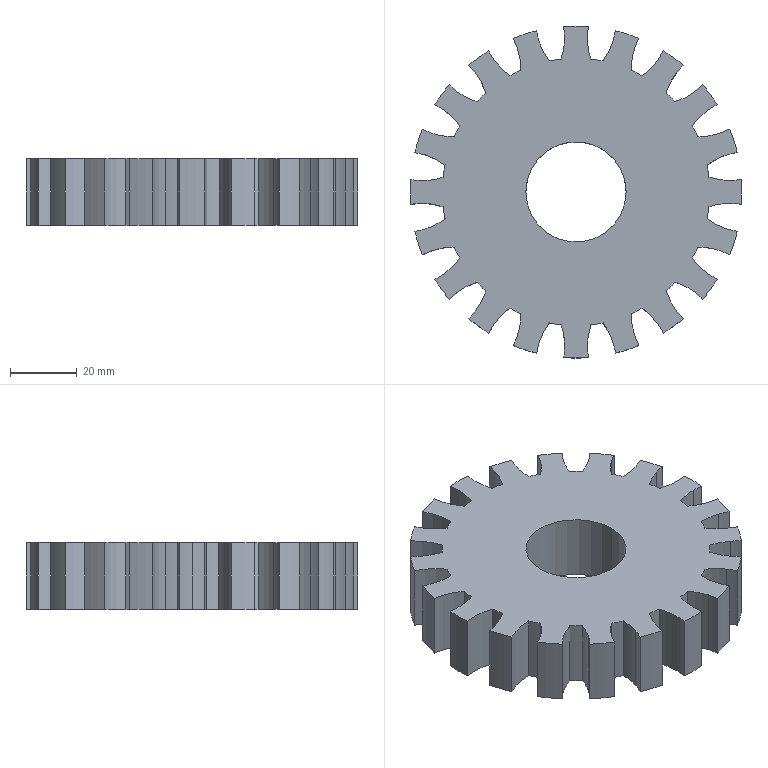Part | SolidWorks | features ICE 2, CirPattern 1, Cut 1, Extrusion 1 | 1 solid | 105 faces | box 99.281 x 99.281 x 20 mm | volume 114594 mm3 | cylinder 103 | plane 2 | commonest cylinder face diameters 40.3 x60 99.281 x21 80 x20 30 x2